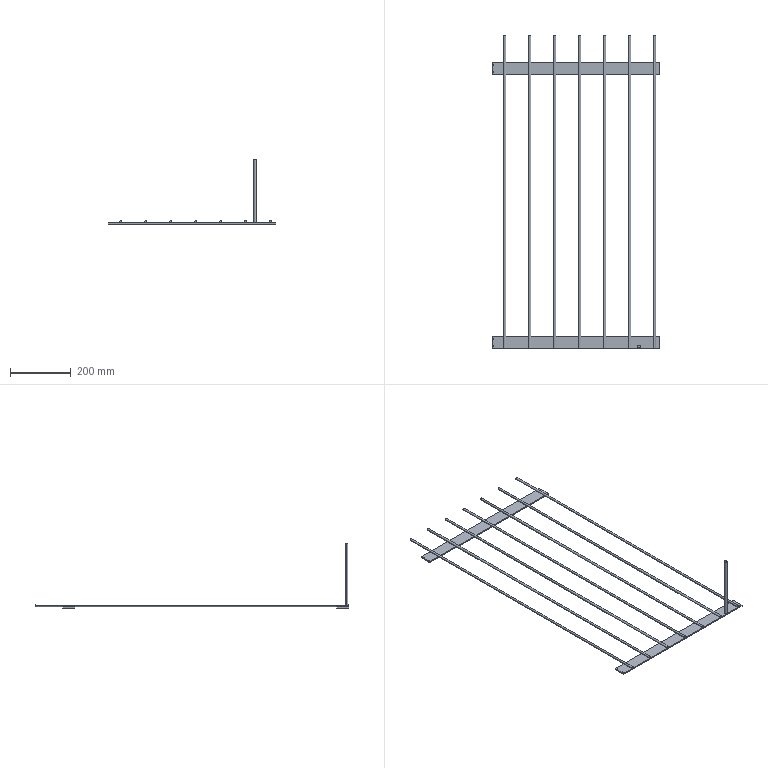Part | STEP file | Guard baffle | 9 solids | 51 faces | box 550 x 1030 x 211 mm | volume 463741 mm3 | plane 27 | cylinder 24 | commonest cylinder face diameters 7 x14 3.3 x8 8 x2